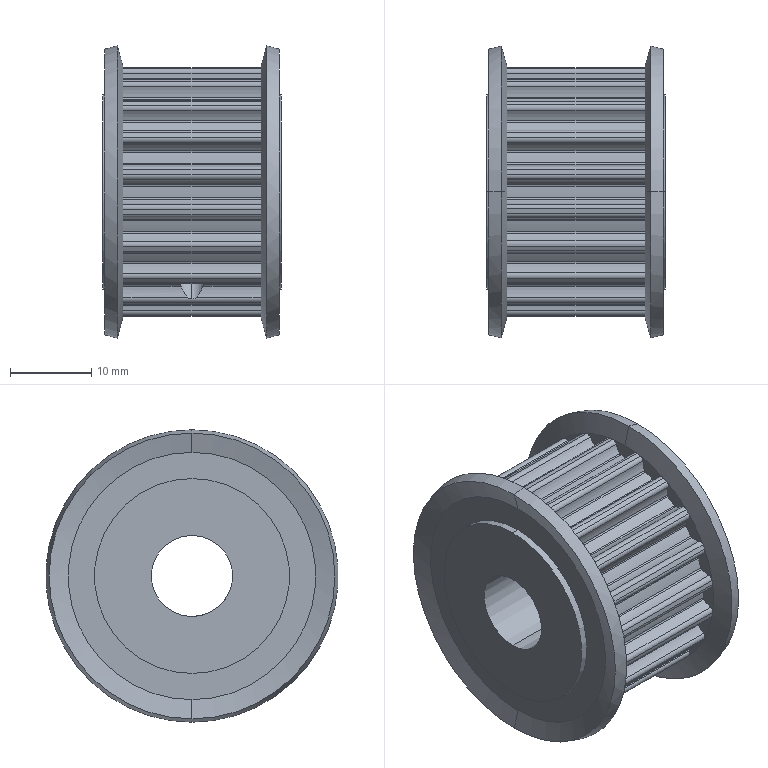Part | SolidWorks | features BaseBody 1 | 1 solid | 236 faces | box 22 x 36 x 36 mm | volume 13261 mm3 | cylinder 180 | plane 44 | cone 12 | commonest cylinder face diameters 0.5 x44 6.55 x44 1.1 x40 27.33 x22 30.87 x20 3.242 x4